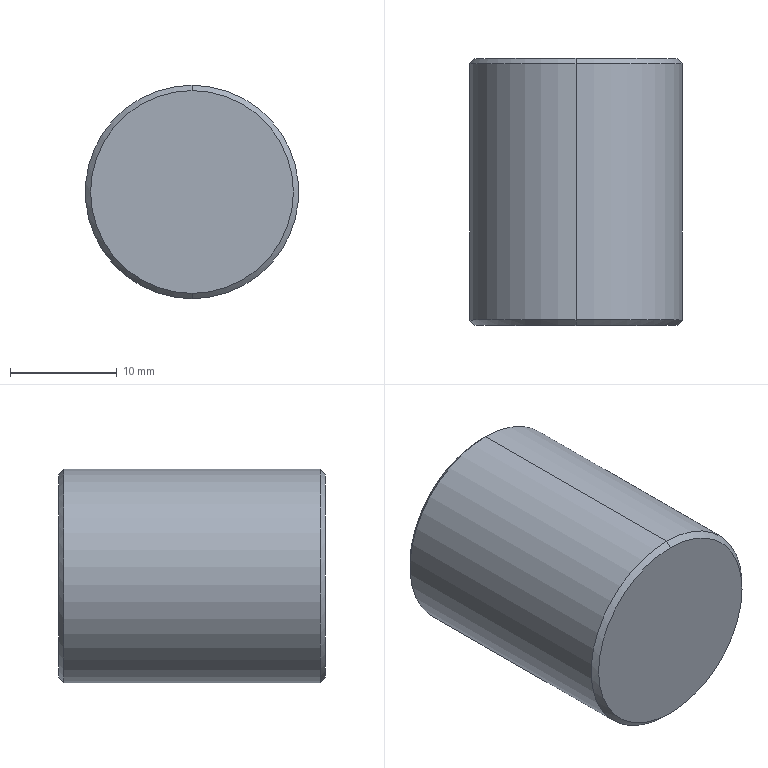Part | NX | features BREP 1 | 1 solid | 11 faces | box 20 x 25 x 20 mm | volume 3862 mm3 | cone 4 | cylinder 4 | plane 3 | commonest cylinder face diameters 15 x2 20 x2
STEP:
#1=CARTESIAN_POINT('',(0.,-12.5,-9.5));
#2=VERTEX_POINT('',#1);
#3=CARTESIAN_POINT('',(0.,-12.5,9.5));
#4=VERTEX_POINT('',#3);
#5=CARTESIAN_POINT('',(0.,-12.5,0.));
#6=DIRECTION('',(0.,-1.,0.));
#7=DIRECTION('',(0.,0.,1.));
#8=AXIS2_PLACEMENT_3D('',#5,#6,#7);
#9=CIRCLE('',#8,9.5);
#10=EDGE_CURVE('',#2,#4,#9,.T.);
#11=ORIENTED_EDGE('',*,*,#10,.F.);
#12=CARTESIAN_POINT('',(0.,-12.,-10.));
#13=VERTEX_POINT('',#12);
#14=CARTESIAN_POINT('',(0.,-12.,-10.));
#15=DIRECTION('',(0.,0.7071,-0.7071));
#16=VECTOR('',#15,1000.);
#17=LINE('',#14,#16);
#18=EDGE_CURVE('',#13,#2,#17,.F.);
#19=ORIENTED_EDGE('',*,*,#18,.F.);
#20=CARTESIAN_POINT('',(0.,-12.,10.));
#21=VERTEX_POINT('',#20);
#22=CARTESIAN_POINT('',(0.,-12.,0.));
#23=DIRECTION('',(0.,1.,0.));
#24=DIRECTION('',(0.,0.,1.));
#25=AXIS2_PLACEMENT_3D('',#22,#23,#24);
#26=CIRCLE('',#25,10.);
#27=EDGE_CURVE('',#21,#13,#26,.T.);
#28=ORIENTED_EDGE('',*,*,#27,.F.);
#29=CARTESIAN_POINT('',(0.,-12.,10.));
#30=DIRECTION('',(0.,0.7071,0.7071));
#31=VECTOR('',#30,1000.);
#32=LINE('',#29,#31);
#33=EDGE_CURVE('',#21,#4,#32,.F.);
#34=ORIENTED_EDGE('',*,*,#33,.T.);
#35=EDGE_LOOP('',(#11,#19,#28,#34));
#36=FACE_BOUND('',#35,.T.);
#37=CARTESIAN_POINT('',(0.,-12.,0.));
#38=DIRECTION('',(0.,1.,0.));
#39=DIRECTION('',(0.,0.,1.));
#40=AXIS2_PLACEMENT_3D('',#37,#38,#39);
#41=CONICAL_SURFACE('',#40,10.,0.7854);
#42=ADVANCED_FACE('',(#36),#41,.T.);
#43=CARTESIAN_POINT('',(0.,12.5,9.5));
#44=VERTEX_POINT('',#43);
#45=CARTESIAN_POINT('',(0.,12.5,-9.5));
#46=VERTEX_POINT('',#45);
#47=CARTESIAN_POINT('',(0.,12.5,0.));
#48=DIRECTION('',(0.,1.,0.));
#49=DIRECTION('',(0.,0.,1.));
#50=AXIS2_PLACEMENT_3D('',#47,#48,#49);
#51=CIRCLE('',#50,9.5);
#52=EDGE_CURVE('',#44,#46,#51,.T.);
#53=ORIENTED_EDGE('',*,*,#52,.F.);
#54=CARTESIAN_POINT('',(0.,12.,10.));
#55=VERTEX_POINT('',#54);
#56=CARTESIAN_POINT('',(0.,12.5,9.5));
#57=DIRECTION('',(0.,-0.7071,0.7071));
#58=VECTOR('',#57,1000.);
#59=LINE('',#56,#58);
#60=EDGE_CURVE('',#44,#55,#59,.T.);
#61=ORIENTED_EDGE('',*,*,#60,.T.);
#62=CARTESIAN_POINT('',(0.,12.,-10.));
#63=VERTEX_POINT('',#62);
#64=CARTESIAN_POINT('',(0.,12.,0.));
#65=DIRECTION('',(0.,-1.,0.));
#66=DIRECTION('',(0.,0.,1.));
#67=AXIS2_PLACEMENT_3D('',#64,#65,#66);
#68=CIRCLE('',#67,10.);
#69=EDGE_CURVE('',#63,#55,#68,.T.);
#70=ORIENTED_EDGE('',*,*,#69,.F.);
#71=CARTESIAN_POINT('',(0.,12.5,-9.5));
#72=DIRECTION('',(0.,-0.7071,-0.7071));
#73=VECTOR('',#72,1000.);
#74=LINE('',#71,#73);
#75=EDGE_CURVE('',#46,#63,#74,.T.);
#76=ORIENTED_EDGE('',*,*,#75,.F.);
#77=EDGE_LOOP('',(#53,#61,#70,#76));
#78=FACE_BOUND('',#77,.T.);
#79=CARTESIAN_POINT('',(0.,12.5,0.));
#80=DIRECTION('',(0.,-1.,0.));
#81=DIRECTION('',(0.,0.,-1.));
#82=AXIS2_PLACEMENT_3D('',#79,#80,#81);
#83=CONICAL_SURFACE('',#82,9.5,0.7854);
#84=ADVANCED_FACE('',(#78),#83,.T.);
#85=CARTESIAN_POINT('',(0.,12.5,-7.5));
#86=VERTEX_POINT('',#85);
#87=CARTESIAN_POINT('',(0.,12.5,7.5));
#88=VERTEX_POINT('',#87);
#89=CARTESIAN_POINT('',(0.,12.5,0.));
#90=DIRECTION('',(0.,1.,0.));
#91=DIRECTION('',(0.,0.,1.));
#92=AXIS2_PLACEMENT_3D('',#89,#90,#91);
#93=CIRCLE('',#92,7.5);
#94=EDGE_CURVE('',#86,#88,#93,.T.);
#95=ORIENTED_EDGE('',*,*,#94,.T.);
#96=CARTESIAN_POINT('',(0.,-10.,7.5));
#97=VERTEX_POINT('',#96);
#98=CARTESIAN_POINT('',(0.,12.5,7.5));
#99=DIRECTION('',(0.,-1.,0.));
#100=VECTOR('',#99,1000.);
#101=LINE('',#98,#100);
#102=EDGE_CURVE('',#88,#97,#101,.T.);
#103=ORIENTED_EDGE('',*,*,#102,.T.);
#104=CARTESIAN_POINT('',(0.,-10.,-7.5));
#105=VERTEX_POINT('',#104);
#106=CARTESIAN_POINT('',(0.,-10.,0.));
#107=DIRECTION('',(0.,1.,0.));
#108=DIRECTION('',(0.,0.,1.));
#109=AXIS2_PLACEMENT_3D('',#106,#107,#108);
#110=CIRCLE('',#109,7.5);
#111=EDGE_CURVE('',#105,#97,#110,.T.);
#112=ORIENTED_EDGE('',*,*,#111,.F.);
#113=CARTESIAN_POINT('',(0.,12.5,-7.5));
#114=DIRECTION('',(0.,-1.,0.));
#115=VECTOR('',#114,1000.);
#116=LINE('',#113,#115);
#117=EDGE_CURVE('',#86,#105,#116,.T.);
#118=ORIENTED_EDGE('',*,*,#117,.F.);
#119=EDGE_LOOP('',(#95,#103,#112,#118));
#120=FACE_BOUND('',#119,.T.);
#121=CARTESIAN_POINT('',(0.,12.5,0.));
#122=DIRECTION('',(0.,-1.,0.));
#123=DIRECTION('',(0.,0.,-1.));
#124=AXIS2_PLACEMENT_3D('',#121,#122,#123);
#125=CYLINDRICAL_SURFACE('',#124,7.5);
#126=ADVANCED_FACE('',(#120),#125,.F.);
#127=ORIENTED_EDGE('',*,*,#69,.T.);
#128=CARTESIAN_POINT('',(0.,12.5,10.));
#129=DIRECTION('',(0.,-1.,0.));
#130=VECTOR('',#129,1000.);
#131=LINE('',#128,#130);
#132=EDGE_CURVE('',#55,#21,#131,.T.);
#133=ORIENTED_EDGE('',*,*,#132,.T.);
#134=ORIENTED_EDGE('',*,*,#27,.T.);
#135=CARTESIAN_POINT('',(0.,12.5,-10.));
#136=DIRECTION('',(0.,-1.,0.));
#137=VECTOR('',#136,1000.);
#138=LINE('',#135,#137);
#139=EDGE_CURVE('',#63,#13,#138,.T.);
#140=ORIENTED_EDGE('',*,*,#139,.F.);
#141=EDGE_LOOP('',(#127,#133,#134,#140));
#142=FACE_BOUND('',#141,.T.);
#143=CARTESIAN_POINT('',(0.,12.5,0.));
#144=DIRECTION('',(0.,-1.,0.));
#145=DIRECTION('',(0.,0.,-1.));
#146=AXIS2_PLACEMENT_3D('',#143,#144,#145);
#147=CYLINDRICAL_SURFACE('',#146,10.);
#148=ADVANCED_FACE('',(#142),#147,.T.);
#149=ORIENTED_EDGE('',*,*,#132,.F.);
#150=CARTESIAN_POINT('',(0.,12.,0.));
#151=DIRECTION('',(0.,-1.,0.));
#152=DIRECTION('',(0.,0.,1.));
#153=AXIS2_PLACEMENT_3D('',#150,#151,#152);
#154=CIRCLE('',#153,10.);
#155=EDGE_CURVE('',#55,#63,#154,.T.);
#156=ORIENTED_EDGE('',*,*,#155,.T.);
#157=ORIENTED_EDGE('',*,*,#139,.T.);
#158=CARTESIAN_POINT('',(0.,-12.,0.));
#159=DIRECTION('',(0.,1.,0.));
#160=DIRECTION('',(0.,0.,1.));
#161=AXIS2_PLACEMENT_3D('',#158,#159,#160);
#162=CIRCLE('',#161,10.);
#163=EDGE_CURVE('',#13,#21,#162,.T.);
#164=ORIENTED_EDGE('',*,*,#163,.T.);
#165=EDGE_LOOP('',(#149,#156,#157,#164));
#166=FACE_BOUND('',#165,.T.);
#167=CARTESIAN_POINT('',(0.,12.5,0.));
#168=DIRECTION('',(0.,-1.,0.));
#169=DIRECTION('',(0.,0.,-1.));
#170=AXIS2_PLACEMENT_3D('',#167,#168,#169);
#171=CYLINDRICAL_SURFACE('',#170,10.);
#172=ADVANCED_FACE('',(#166),#171,.T.);
#173=CARTESIAN_POINT('',(0.,12.5,0.));
#174=DIRECTION('',(0.,1.,0.));
#175=DIRECTION('',(0.,0.,1.));
#176=AXIS2_PLACEMENT_3D('',#173,#174,#175);
#177=CIRCLE('',#176,9.5);
#178=EDGE_CURVE('',#46,#44,#177,.T.);
#179=ORIENTED_EDGE('',*,*,#178,.T.);
#180=ORIENTED_EDGE('',*,*,#52,.T.);
#181=EDGE_LOOP('',(#179,#180));
#182=FACE_BOUND('',#181,.T.);
#183=ORIENTED_EDGE('',*,*,#94,.F.);
#184=CARTESIAN_POINT('',(0.,12.5,0.));
#185=DIRECTION('',(0.,1.,0.));
#186=DIRECTION('',(0.,0.,1.));
#187=AXIS2_PLACEMENT_3D('',#184,#185,#186);
#188=CIRCLE('',#187,7.5);
#189=EDGE_CURVE('',#88,#86,#188,.T.);
#190=ORIENTED_EDGE('',*,*,#189,.F.);
#191=EDGE_LOOP('',(#183,#190));
#192=FACE_BOUND('',#191,.T.);
#193=CARTESIAN_POINT('',(0.,12.5,0.));
#194=DIRECTION('',(0.,1.,0.));
#195=DIRECTION('',(1.,0.,0.));
#196=AXIS2_PLACEMENT_3D('',#193,#194,#195);
#197=PLANE('',#196);
#198=ADVANCED_FACE('',(#182,#192),#197,.T.);
#199=CARTESIAN_POINT('',(0.,-12.5,0.));
#200=DIRECTION('',(0.,-1.,0.));
#201=DIRECTION('',(0.,0.,1.));
#202=AXIS2_PLACEMENT_3D('',#199,#200,#201);
#203=CIRCLE('',#202,9.5);
#204=EDGE_CURVE('',#4,#2,#203,.T.);
#205=ORIENTED_EDGE('',*,*,#204,.T.);
#206=ORIENTED_EDGE('',*,*,#10,.T.);
#207=EDGE_LOOP('',(#205,#206));
#208=FACE_BOUND('',#207,.T.);
#209=CARTESIAN_POINT('',(0.,-12.5,0.));
#210=DIRECTION('',(0.,1.,0.));
#211=DIRECTION('',(1.,0.,0.));
#212=AXIS2_PLACEMENT_3D('',#209,#210,#211);
#213=PLANE('',#212);
#214=ADVANCED_FACE('',(#208),#213,.F.);
#215=ORIENTED_EDGE('',*,*,#102,.F.);
#216=ORIENTED_EDGE('',*,*,#189,.T.);
#217=ORIENTED_EDGE('',*,*,#117,.T.);
#218=CARTESIAN_POINT('',(0.,-10.,0.));
#219=DIRECTION('',(0.,1.,0.));
#220=DIRECTION('',(0.,0.,1.));
#221=AXIS2_PLACEMENT_3D('',#218,#219,#220);
#222=CIRCLE('',#221,7.5);
#223=EDGE_CURVE('',#97,#105,#222,.T.);
#224=ORIENTED_EDGE('',*,*,#223,.F.);
#225=EDGE_LOOP('',(#215,#216,#217,#224));
#226=FACE_BOUND('',#225,.T.);
#227=CARTESIAN_POINT('',(0.,12.5,0.));
#228=DIRECTION('',(0.,-1.,0.));
#229=DIRECTION('',(0.,0.,-1.));
#230=AXIS2_PLACEMENT_3D('',#227,#228,#229);
#231=CYLINDRICAL_SURFACE('',#230,7.5);
#232=ADVANCED_FACE('',(#226),#231,.F.);
#233=ORIENTED_EDGE('',*,*,#111,.T.);
#234=ORIENTED_EDGE('',*,*,#223,.T.);
#235=EDGE_LOOP('',(#233,#234));
#236=FACE_BOUND('',#235,.T.);
#237=CARTESIAN_POINT('',(0.,-10.,0.));
#238=DIRECTION('',(0.,1.,0.));
#239=DIRECTION('',(1.,0.,0.));
#240=AXIS2_PLACEMENT_3D('',#237,#238,#239);
#241=PLANE('',#240);
#242=ADVANCED_FACE('',(#236),#241,.T.);
#243=ORIENTED_EDGE('',*,*,#60,.F.);
#244=ORIENTED_EDGE('',*,*,#178,.F.);
#245=ORIENTED_EDGE('',*,*,#75,.T.);
#246=ORIENTED_EDGE('',*,*,#155,.F.);
#247=EDGE_LOOP('',(#243,#244,#245,#246));
#248=FACE_BOUND('',#247,.T.);
#249=CARTESIAN_POINT('',(0.,12.5,0.));
#250=DIRECTION('',(0.,-1.,0.));
#251=DIRECTION('',(0.,0.,-1.));
#252=AXIS2_PLACEMENT_3D('',#249,#250,#251);
#253=CONICAL_SURFACE('',#252,9.5,0.7854);
#254=ADVANCED_FACE('',(#248),#253,.T.);
#255=ORIENTED_EDGE('',*,*,#18,.T.);
#256=ORIENTED_EDGE('',*,*,#204,.F.);
#257=ORIENTED_EDGE('',*,*,#33,.F.);
#258=ORIENTED_EDGE('',*,*,#163,.F.);
#259=EDGE_LOOP('',(#255,#256,#257,#258));
#260=FACE_BOUND('',#259,.T.);
#261=CARTESIAN_POINT('',(0.,-12.,0.));
#262=DIRECTION('',(0.,1.,0.));
#263=DIRECTION('',(0.,0.,1.));
#264=AXIS2_PLACEMENT_3D('',#261,#262,#263);
#265=CONICAL_SURFACE('',#264,10.,0.7854);
#266=ADVANCED_FACE('',(#260),#265,.T.);
#267=CLOSED_SHELL('',(#42,#84,#126,#148,#172,#198,#214,#232,#242,#254,#266));
#268=MANIFOLD_SOLID_BREP('',#267);
#269=(LENGTH_UNIT()NAMED_UNIT(*)SI_UNIT(.MILLI.,.METRE.));
#270=UNCERTAINTY_MEASURE_WITH_UNIT(LENGTH_MEASURE(0.00001),#269,'','');
#271=(NAMED_UNIT(*)PLANE_ANGLE_UNIT()SI_UNIT($,.RADIAN.));
#272=(NAMED_UNIT(*)SI_UNIT($,.STERADIAN.)SOLID_ANGLE_UNIT());
#273=(GEOMETRIC_REPRESENTATION_CONTEXT(3)GLOBAL_UNCERTAINTY_ASSIGNED_CONTEXT((#270))GLOBAL_UNIT_ASSIGNED_CONTEXT((#269,#271,#272))REPRESENTATION_CONTEXT('',''));
#274=ADVANCED_BREP_SHAPE_REPRESENTATION('',(#268),#273);